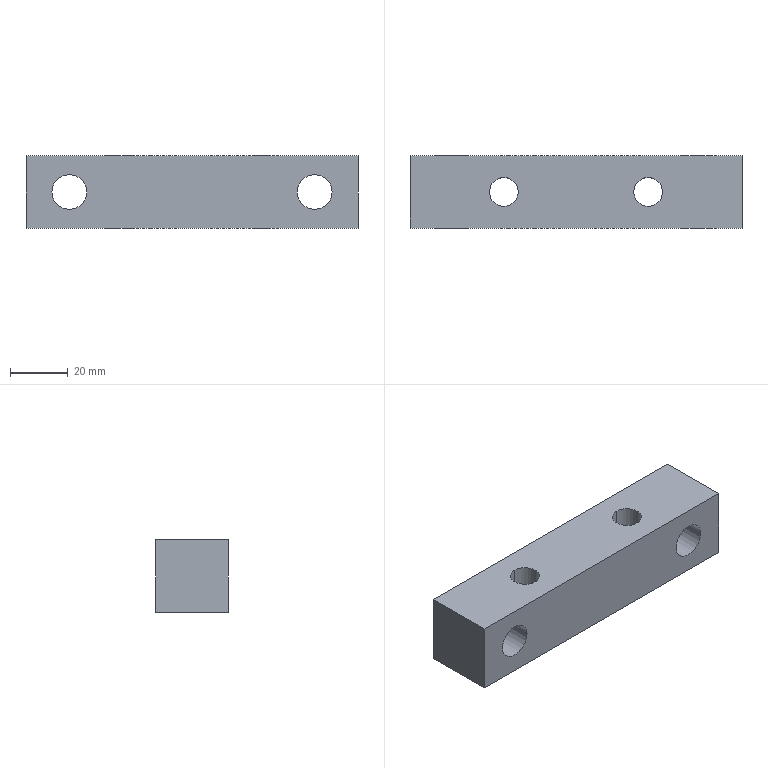Part | STEP file | J205-EBZ05-05-35 | 1 solid | 14 faces | box 115 x 25 x 25 mm | volume 62293 mm3 | cylinder 8 | plane 6 | commonest cylinder face diameters 10 x4 12 x4
STEP:
#1=CARTESIAN_POINT('',(84.,25.,12.5));
#2=VERTEX_POINT('',#1);
#3=CARTESIAN_POINT('',(96.,25.,12.5));
#4=VERTEX_POINT('',#3);
#5=CARTESIAN_POINT('',(90.,25.,12.5));
#6=DIRECTION('',(0.,-1.,0.));
#7=DIRECTION('',(1.,0.,0.));
#8=AXIS2_PLACEMENT_3D('',#5,#6,#7);
#9=CIRCLE('',#8,6.);
#10=EDGE_CURVE('',#2,#4,#9,.T.);
#11=ORIENTED_EDGE('',*,*,#10,.F.);
#12=CARTESIAN_POINT('',(84.,0.,12.5));
#13=VERTEX_POINT('',#12);
#14=CARTESIAN_POINT('',(84.,25.,12.5));
#15=DIRECTION('',(0.,-1.,0.));
#16=VECTOR('',#15,1000.);
#17=LINE('',#14,#16);
#18=EDGE_CURVE('',#2,#13,#17,.T.);
#19=ORIENTED_EDGE('',*,*,#18,.T.);
#20=CARTESIAN_POINT('',(96.,0.,12.5));
#21=VERTEX_POINT('',#20);
#22=CARTESIAN_POINT('',(90.,0.,12.5));
#23=DIRECTION('',(0.,1.,0.));
#24=DIRECTION('',(-1.,0.,0.));
#25=AXIS2_PLACEMENT_3D('',#22,#23,#24);
#26=CIRCLE('',#25,6.);
#27=EDGE_CURVE('',#21,#13,#26,.T.);
#28=ORIENTED_EDGE('',*,*,#27,.F.);
#29=CARTESIAN_POINT('',(96.,25.,12.5));
#30=DIRECTION('',(0.,-1.,0.));
#31=VECTOR('',#30,1000.);
#32=LINE('',#29,#31);
#33=EDGE_CURVE('',#4,#21,#32,.T.);
#34=ORIENTED_EDGE('',*,*,#33,.F.);
#35=EDGE_LOOP('',(#11,#19,#28,#34));
#36=FACE_OUTER_BOUND('',#35,.T.);
#37=CARTESIAN_POINT('',(90.,25.,12.5));
#38=DIRECTION('',(0.,-1.,0.));
#39=DIRECTION('',(1.,0.,0.));
#40=AXIS2_PLACEMENT_3D('',#37,#38,#39);
#41=CYLINDRICAL_SURFACE('',#40,6.);
#42=ADVANCED_FACE('',(#36),#41,.F.);
#43=CARTESIAN_POINT('',(-1.,25.,12.5));
#44=VERTEX_POINT('',#43);
#45=CARTESIAN_POINT('',(11.,25.,12.5));
#46=VERTEX_POINT('',#45);
#47=CARTESIAN_POINT('',(5.,25.,12.5));
#48=DIRECTION('',(0.,-1.,0.));
#49=DIRECTION('',(1.,0.,0.));
#50=AXIS2_PLACEMENT_3D('',#47,#48,#49);
#51=CIRCLE('',#50,6.);
#52=EDGE_CURVE('',#44,#46,#51,.T.);
#53=ORIENTED_EDGE('',*,*,#52,.F.);
#54=CARTESIAN_POINT('',(-1.,0.,12.5));
#55=VERTEX_POINT('',#54);
#56=CARTESIAN_POINT('',(-1.,25.,12.5));
#57=DIRECTION('',(0.,-1.,0.));
#58=VECTOR('',#57,1000.);
#59=LINE('',#56,#58);
#60=EDGE_CURVE('',#44,#55,#59,.T.);
#61=ORIENTED_EDGE('',*,*,#60,.T.);
#62=CARTESIAN_POINT('',(11.,0.,12.5));
#63=VERTEX_POINT('',#62);
#64=CARTESIAN_POINT('',(5.,0.,12.5));
#65=DIRECTION('',(0.,1.,0.));
#66=DIRECTION('',(-1.,0.,0.));
#67=AXIS2_PLACEMENT_3D('',#64,#65,#66);
#68=CIRCLE('',#67,6.);
#69=EDGE_CURVE('',#63,#55,#68,.T.);
#70=ORIENTED_EDGE('',*,*,#69,.F.);
#71=CARTESIAN_POINT('',(11.,25.,12.5));
#72=DIRECTION('',(0.,-1.,0.));
#73=VECTOR('',#72,1000.);
#74=LINE('',#71,#73);
#75=EDGE_CURVE('',#46,#63,#74,.T.);
#76=ORIENTED_EDGE('',*,*,#75,.F.);
#77=EDGE_LOOP('',(#53,#61,#70,#76));
#78=FACE_OUTER_BOUND('',#77,.T.);
#79=CARTESIAN_POINT('',(5.,25.,12.5));
#80=DIRECTION('',(0.,-1.,0.));
#81=DIRECTION('',(1.,0.,0.));
#82=AXIS2_PLACEMENT_3D('',#79,#80,#81);
#83=CYLINDRICAL_SURFACE('',#82,6.);
#84=ADVANCED_FACE('',(#78),#83,.F.);
#85=CARTESIAN_POINT('',(22.5,17.5,25.));
#86=VERTEX_POINT('',#85);
#87=CARTESIAN_POINT('',(22.5,7.5,25.));
#88=VERTEX_POINT('',#87);
#89=CARTESIAN_POINT('',(22.5,12.5,25.));
#90=DIRECTION('',(0.,0.,-1.));
#91=DIRECTION('',(0.,-1.,0.));
#92=AXIS2_PLACEMENT_3D('',#89,#90,#91);
#93=CIRCLE('',#92,5.);
#94=EDGE_CURVE('',#86,#88,#93,.T.);
#95=ORIENTED_EDGE('',*,*,#94,.F.);
#96=CARTESIAN_POINT('',(22.5,17.5,0.));
#97=VERTEX_POINT('',#96);
#98=CARTESIAN_POINT('',(22.5,17.5,25.));
#99=DIRECTION('',(0.,0.,-1.));
#100=VECTOR('',#99,1000.);
#101=LINE('',#98,#100);
#102=EDGE_CURVE('',#86,#97,#101,.T.);
#103=ORIENTED_EDGE('',*,*,#102,.T.);
#104=CARTESIAN_POINT('',(22.5,7.5,0.));
#105=VERTEX_POINT('',#104);
#106=CARTESIAN_POINT('',(22.5,12.5,0.));
#107=DIRECTION('',(0.,0.,1.));
#108=DIRECTION('',(0.,1.,0.));
#109=AXIS2_PLACEMENT_3D('',#106,#107,#108);
#110=CIRCLE('',#109,5.);
#111=EDGE_CURVE('',#105,#97,#110,.T.);
#112=ORIENTED_EDGE('',*,*,#111,.F.);
#113=CARTESIAN_POINT('',(22.5,7.5,25.));
#114=DIRECTION('',(0.,0.,-1.));
#115=VECTOR('',#114,1000.);
#116=LINE('',#113,#115);
#117=EDGE_CURVE('',#88,#105,#116,.T.);
#118=ORIENTED_EDGE('',*,*,#117,.F.);
#119=EDGE_LOOP('',(#95,#103,#112,#118));
#120=FACE_OUTER_BOUND('',#119,.T.);
#121=CARTESIAN_POINT('',(22.5,12.5,25.));
#122=DIRECTION('',(0.,0.,-1.));
#123=DIRECTION('',(0.,-1.,0.));
#124=AXIS2_PLACEMENT_3D('',#121,#122,#123);
#125=CYLINDRICAL_SURFACE('',#124,5.);
#126=ADVANCED_FACE('',(#120),#125,.F.);
#127=CARTESIAN_POINT('',(72.5,17.5,25.));
#128=VERTEX_POINT('',#127);
#129=CARTESIAN_POINT('',(72.5,7.5,25.));
#130=VERTEX_POINT('',#129);
#131=CARTESIAN_POINT('',(72.5,12.5,25.));
#132=DIRECTION('',(0.,0.,-1.));
#133=DIRECTION('',(0.,-1.,0.));
#134=AXIS2_PLACEMENT_3D('',#131,#132,#133);
#135=CIRCLE('',#134,5.);
#136=EDGE_CURVE('',#128,#130,#135,.T.);
#137=ORIENTED_EDGE('',*,*,#136,.F.);
#138=CARTESIAN_POINT('',(72.5,17.5,0.));
#139=VERTEX_POINT('',#138);
#140=CARTESIAN_POINT('',(72.5,17.5,25.));
#141=DIRECTION('',(0.,0.,-1.));
#142=VECTOR('',#141,1000.);
#143=LINE('',#140,#142);
#144=EDGE_CURVE('',#128,#139,#143,.T.);
#145=ORIENTED_EDGE('',*,*,#144,.T.);
#146=CARTESIAN_POINT('',(72.5,7.5,0.));
#147=VERTEX_POINT('',#146);
#148=CARTESIAN_POINT('',(72.5,12.5,0.));
#149=DIRECTION('',(0.,0.,1.));
#150=DIRECTION('',(0.,1.,0.));
#151=AXIS2_PLACEMENT_3D('',#148,#149,#150);
#152=CIRCLE('',#151,5.);
#153=EDGE_CURVE('',#147,#139,#152,.T.);
#154=ORIENTED_EDGE('',*,*,#153,.F.);
#155=CARTESIAN_POINT('',(72.5,7.5,25.));
#156=DIRECTION('',(0.,0.,-1.));
#157=VECTOR('',#156,1000.);
#158=LINE('',#155,#157);
#159=EDGE_CURVE('',#130,#147,#158,.T.);
#160=ORIENTED_EDGE('',*,*,#159,.F.);
#161=EDGE_LOOP('',(#137,#145,#154,#160));
#162=FACE_OUTER_BOUND('',#161,.T.);
#163=CARTESIAN_POINT('',(72.5,12.5,25.));
#164=DIRECTION('',(0.,0.,-1.));
#165=DIRECTION('',(0.,-1.,0.));
#166=AXIS2_PLACEMENT_3D('',#163,#164,#165);
#167=CYLINDRICAL_SURFACE('',#166,5.);
#168=ADVANCED_FACE('',(#162),#167,.F.);
#169=CARTESIAN_POINT('',(90.,25.,12.5));
#170=DIRECTION('',(0.,-1.,0.));
#171=DIRECTION('',(1.,0.,0.));
#172=AXIS2_PLACEMENT_3D('',#169,#170,#171);
#173=CIRCLE('',#172,6.);
#174=EDGE_CURVE('',#4,#2,#173,.T.);
#175=ORIENTED_EDGE('',*,*,#174,.T.);
#176=ORIENTED_EDGE('',*,*,#10,.T.);
#177=EDGE_LOOP('',(#175,#176));
#178=FACE_BOUND('',#177,.T.);
#179=CARTESIAN_POINT('',(5.,25.,12.5));
#180=DIRECTION('',(0.,-1.,0.));
#181=DIRECTION('',(1.,0.,0.));
#182=AXIS2_PLACEMENT_3D('',#179,#180,#181);
#183=CIRCLE('',#182,6.);
#184=EDGE_CURVE('',#46,#44,#183,.T.);
#185=ORIENTED_EDGE('',*,*,#184,.T.);
#186=ORIENTED_EDGE('',*,*,#52,.T.);
#187=EDGE_LOOP('',(#185,#186));
#188=FACE_BOUND('',#187,.T.);
#189=CARTESIAN_POINT('',(-10.,25.,0.));
#190=VERTEX_POINT('',#189);
#191=CARTESIAN_POINT('',(105.,25.,0.));
#192=VERTEX_POINT('',#191);
#193=CARTESIAN_POINT('',(47.5,25.,0.));
#194=DIRECTION('',(1.,0.,0.));
#195=VECTOR('',#194,1000.);
#196=LINE('',#193,#195);
#197=EDGE_CURVE('',#190,#192,#196,.T.);
#198=ORIENTED_EDGE('',*,*,#197,.F.);
#199=CARTESIAN_POINT('',(-10.,25.,25.));
#200=VERTEX_POINT('',#199);
#201=CARTESIAN_POINT('',(-10.,25.,12.5));
#202=DIRECTION('',(0.,0.,-1.));
#203=VECTOR('',#202,1000.);
#204=LINE('',#201,#203);
#205=EDGE_CURVE('',#200,#190,#204,.T.);
#206=ORIENTED_EDGE('',*,*,#205,.F.);
#207=CARTESIAN_POINT('',(105.,25.,25.));
#208=VERTEX_POINT('',#207);
#209=CARTESIAN_POINT('',(47.5,25.,25.));
#210=DIRECTION('',(-1.,0.,0.));
#211=VECTOR('',#210,1000.);
#212=LINE('',#209,#211);
#213=EDGE_CURVE('',#208,#200,#212,.T.);
#214=ORIENTED_EDGE('',*,*,#213,.F.);
#215=CARTESIAN_POINT('',(105.,25.,12.5));
#216=DIRECTION('',(0.,0.,1.));
#217=VECTOR('',#216,1000.);
#218=LINE('',#215,#217);
#219=EDGE_CURVE('',#192,#208,#218,.T.);
#220=ORIENTED_EDGE('',*,*,#219,.F.);
#221=EDGE_LOOP('',(#198,#206,#214,#220));
#222=FACE_OUTER_BOUND('',#221,.T.);
#223=CARTESIAN_POINT('',(47.5,25.,12.5));
#224=DIRECTION('',(0.,1.,0.));
#225=DIRECTION('',(-1.,0.,0.));
#226=AXIS2_PLACEMENT_3D('',#223,#224,#225);
#227=PLANE('',#226);
#228=ADVANCED_FACE('',(#178,#188,#222),#227,.T.);
#229=ORIENTED_EDGE('',*,*,#111,.T.);
#230=CARTESIAN_POINT('',(22.5,12.5,0.));
#231=DIRECTION('',(0.,0.,1.));
#232=DIRECTION('',(0.,1.,0.));
#233=AXIS2_PLACEMENT_3D('',#230,#231,#232);
#234=CIRCLE('',#233,5.);
#235=EDGE_CURVE('',#97,#105,#234,.T.);
#236=ORIENTED_EDGE('',*,*,#235,.T.);
#237=EDGE_LOOP('',(#229,#236));
#238=FACE_BOUND('',#237,.T.);
#239=ORIENTED_EDGE('',*,*,#153,.T.);
#240=CARTESIAN_POINT('',(72.5,12.5,0.));
#241=DIRECTION('',(0.,0.,1.));
#242=DIRECTION('',(0.,1.,0.));
#243=AXIS2_PLACEMENT_3D('',#240,#241,#242);
#244=CIRCLE('',#243,5.);
#245=EDGE_CURVE('',#139,#147,#244,.T.);
#246=ORIENTED_EDGE('',*,*,#245,.T.);
#247=EDGE_LOOP('',(#239,#246));
#248=FACE_BOUND('',#247,.T.);
#249=CARTESIAN_POINT('',(-10.,0.,0.));
#250=VERTEX_POINT('',#249);
#251=CARTESIAN_POINT('',(-10.,0.,0.));
#252=DIRECTION('',(0.,1.,0.));
#253=VECTOR('',#252,1000.);
#254=LINE('',#251,#253);
#255=EDGE_CURVE('',#250,#190,#254,.T.);
#256=ORIENTED_EDGE('',*,*,#255,.T.);
#257=ORIENTED_EDGE('',*,*,#197,.T.);
#258=CARTESIAN_POINT('',(105.,0.,0.));
#259=VERTEX_POINT('',#258);
#260=CARTESIAN_POINT('',(105.,0.,0.));
#261=DIRECTION('',(0.,1.,0.));
#262=VECTOR('',#261,1000.);
#263=LINE('',#260,#262);
#264=EDGE_CURVE('',#259,#192,#263,.T.);
#265=ORIENTED_EDGE('',*,*,#264,.F.);
#266=CARTESIAN_POINT('',(47.5,0.,0.));
#267=DIRECTION('',(-1.,0.,0.));
#268=VECTOR('',#267,1000.);
#269=LINE('',#266,#268);
#270=EDGE_CURVE('',#259,#250,#269,.T.);
#271=ORIENTED_EDGE('',*,*,#270,.T.);
#272=EDGE_LOOP('',(#256,#257,#265,#271));
#273=FACE_OUTER_BOUND('',#272,.T.);
#274=CARTESIAN_POINT('',(47.5,0.,0.));
#275=DIRECTION('',(0.,0.,-1.));
#276=DIRECTION('',(0.,-1.,0.));
#277=AXIS2_PLACEMENT_3D('',#274,#275,#276);
#278=PLANE('',#277);
#279=ADVANCED_FACE('',(#238,#248,#273),#278,.T.);
#280=ORIENTED_EDGE('',*,*,#264,.T.);
#281=ORIENTED_EDGE('',*,*,#219,.T.);
#282=CARTESIAN_POINT('',(105.,0.,25.));
#283=VERTEX_POINT('',#282);
#284=CARTESIAN_POINT('',(105.,0.,25.));
#285=DIRECTION('',(0.,1.,0.));
#286=VECTOR('',#285,1000.);
#287=LINE('',#284,#286);
#288=EDGE_CURVE('',#283,#208,#287,.T.);
#289=ORIENTED_EDGE('',*,*,#288,.F.);
#290=CARTESIAN_POINT('',(105.,0.,12.5));
#291=DIRECTION('',(0.,0.,-1.));
#292=VECTOR('',#291,1000.);
#293=LINE('',#290,#292);
#294=EDGE_CURVE('',#283,#259,#293,.T.);
#295=ORIENTED_EDGE('',*,*,#294,.T.);
#296=EDGE_LOOP('',(#280,#281,#289,#295));
#297=FACE_OUTER_BOUND('',#296,.T.);
#298=CARTESIAN_POINT('',(105.,0.,12.5));
#299=DIRECTION('',(1.,0.,0.));
#300=DIRECTION('',(0.,1.,0.));
#301=AXIS2_PLACEMENT_3D('',#298,#299,#300);
#302=PLANE('',#301);
#303=ADVANCED_FACE('',(#297),#302,.T.);
#304=CARTESIAN_POINT('',(22.5,12.5,25.));
#305=DIRECTION('',(0.,0.,-1.));
#306=DIRECTION('',(0.,-1.,0.));
#307=AXIS2_PLACEMENT_3D('',#304,#305,#306);
#308=CIRCLE('',#307,5.);
#309=EDGE_CURVE('',#88,#86,#308,.T.);
#310=ORIENTED_EDGE('',*,*,#309,.T.);
#311=ORIENTED_EDGE('',*,*,#94,.T.);
#312=EDGE_LOOP('',(#310,#311));
#313=FACE_BOUND('',#312,.T.);
#314=CARTESIAN_POINT('',(72.5,12.5,25.));
#315=DIRECTION('',(0.,0.,-1.));
#316=DIRECTION('',(0.,-1.,0.));
#317=AXIS2_PLACEMENT_3D('',#314,#315,#316);
#318=CIRCLE('',#317,5.);
#319=EDGE_CURVE('',#130,#128,#318,.T.);
#320=ORIENTED_EDGE('',*,*,#319,.T.);
#321=ORIENTED_EDGE('',*,*,#136,.T.);
#322=EDGE_LOOP('',(#320,#321));
#323=FACE_BOUND('',#322,.T.);
#324=ORIENTED_EDGE('',*,*,#288,.T.);
#325=ORIENTED_EDGE('',*,*,#213,.T.);
#326=CARTESIAN_POINT('',(-10.,0.,25.));
#327=VERTEX_POINT('',#326);
#328=CARTESIAN_POINT('',(-10.,0.,25.));
#329=DIRECTION('',(0.,1.,0.));
#330=VECTOR('',#329,1000.);
#331=LINE('',#328,#330);
#332=EDGE_CURVE('',#327,#200,#331,.T.);
#333=ORIENTED_EDGE('',*,*,#332,.F.);
#334=CARTESIAN_POINT('',(47.5,0.,25.));
#335=DIRECTION('',(1.,0.,0.));
#336=VECTOR('',#335,1000.);
#337=LINE('',#334,#336);
#338=EDGE_CURVE('',#327,#283,#337,.T.);
#339=ORIENTED_EDGE('',*,*,#338,.T.);
#340=EDGE_LOOP('',(#324,#325,#333,#339));
#341=FACE_OUTER_BOUND('',#340,.T.);
#342=CARTESIAN_POINT('',(47.5,0.,25.));
#343=DIRECTION('',(0.,0.,1.));
#344=DIRECTION('',(0.,1.,0.));
#345=AXIS2_PLACEMENT_3D('',#342,#343,#344);
#346=PLANE('',#345);
#347=ADVANCED_FACE('',(#313,#323,#341),#346,.T.);
#348=ORIENTED_EDGE('',*,*,#27,.T.);
#349=CARTESIAN_POINT('',(90.,0.,12.5));
#350=DIRECTION('',(0.,1.,0.));
#351=DIRECTION('',(-1.,0.,0.));
#352=AXIS2_PLACEMENT_3D('',#349,#350,#351);
#353=CIRCLE('',#352,6.);
#354=EDGE_CURVE('',#13,#21,#353,.T.);
#355=ORIENTED_EDGE('',*,*,#354,.T.);
#356=EDGE_LOOP('',(#348,#355));
#357=FACE_BOUND('',#356,.T.);
#358=ORIENTED_EDGE('',*,*,#69,.T.);
#359=CARTESIAN_POINT('',(5.,0.,12.5));
#360=DIRECTION('',(0.,1.,0.));
#361=DIRECTION('',(-1.,0.,0.));
#362=AXIS2_PLACEMENT_3D('',#359,#360,#361);
#363=CIRCLE('',#362,6.);
#364=EDGE_CURVE('',#55,#63,#363,.T.);
#365=ORIENTED_EDGE('',*,*,#364,.T.);
#366=EDGE_LOOP('',(#358,#365));
#367=FACE_BOUND('',#366,.T.);
#368=CARTESIAN_POINT('',(-10.,0.,12.5));
#369=DIRECTION('',(0.,0.,1.));
#370=VECTOR('',#369,1000.);
#371=LINE('',#368,#370);
#372=EDGE_CURVE('',#250,#327,#371,.T.);
#373=ORIENTED_EDGE('',*,*,#372,.F.);
#374=ORIENTED_EDGE('',*,*,#270,.F.);
#375=ORIENTED_EDGE('',*,*,#294,.F.);
#376=ORIENTED_EDGE('',*,*,#338,.F.);
#377=EDGE_LOOP('',(#373,#374,#375,#376));
#378=FACE_OUTER_BOUND('',#377,.T.);
#379=CARTESIAN_POINT('',(47.5,0.,12.5));
#380=DIRECTION('',(0.,-1.,0.));
#381=DIRECTION('',(1.,0.,0.));
#382=AXIS2_PLACEMENT_3D('',#379,#380,#381);
#383=PLANE('',#382);
#384=ADVANCED_FACE('',(#357,#367,#378),#383,.T.);
#385=ORIENTED_EDGE('',*,*,#372,.T.);
#386=ORIENTED_EDGE('',*,*,#332,.T.);
#387=ORIENTED_EDGE('',*,*,#205,.T.);
#388=ORIENTED_EDGE('',*,*,#255,.F.);
#389=EDGE_LOOP('',(#385,#386,#387,#388));
#390=FACE_OUTER_BOUND('',#389,.T.);
#391=CARTESIAN_POINT('',(-10.,0.,12.5));
#392=DIRECTION('',(-1.,0.,0.));
#393=DIRECTION('',(0.,-1.,0.));
#394=AXIS2_PLACEMENT_3D('',#391,#392,#393);
#395=PLANE('',#394);
#396=ADVANCED_FACE('',(#390),#395,.T.);
#397=ORIENTED_EDGE('',*,*,#144,.F.);
#398=ORIENTED_EDGE('',*,*,#319,.F.);
#399=ORIENTED_EDGE('',*,*,#159,.T.);
#400=ORIENTED_EDGE('',*,*,#245,.F.);
#401=EDGE_LOOP('',(#397,#398,#399,#400));
#402=FACE_OUTER_BOUND('',#401,.T.);
#403=CARTESIAN_POINT('',(72.5,12.5,25.));
#404=DIRECTION('',(0.,0.,-1.));
#405=DIRECTION('',(0.,-1.,0.));
#406=AXIS2_PLACEMENT_3D('',#403,#404,#405);
#407=CYLINDRICAL_SURFACE('',#406,5.);
#408=ADVANCED_FACE('',(#402),#407,.F.);
#409=ORIENTED_EDGE('',*,*,#102,.F.);
#410=ORIENTED_EDGE('',*,*,#309,.F.);
#411=ORIENTED_EDGE('',*,*,#117,.T.);
#412=ORIENTED_EDGE('',*,*,#235,.F.);
#413=EDGE_LOOP('',(#409,#410,#411,#412));
#414=FACE_OUTER_BOUND('',#413,.T.);
#415=CARTESIAN_POINT('',(22.5,12.5,25.));
#416=DIRECTION('',(0.,0.,-1.));
#417=DIRECTION('',(0.,-1.,0.));
#418=AXIS2_PLACEMENT_3D('',#415,#416,#417);
#419=CYLINDRICAL_SURFACE('',#418,5.);
#420=ADVANCED_FACE('',(#414),#419,.F.);
#421=ORIENTED_EDGE('',*,*,#60,.F.);
#422=ORIENTED_EDGE('',*,*,#184,.F.);
#423=ORIENTED_EDGE('',*,*,#75,.T.);
#424=ORIENTED_EDGE('',*,*,#364,.F.);
#425=EDGE_LOOP('',(#421,#422,#423,#424));
#426=FACE_OUTER_BOUND('',#425,.T.);
#427=CARTESIAN_POINT('',(5.,25.,12.5));
#428=DIRECTION('',(0.,-1.,0.));
#429=DIRECTION('',(1.,0.,0.));
#430=AXIS2_PLACEMENT_3D('',#427,#428,#429);
#431=CYLINDRICAL_SURFACE('',#430,6.);
#432=ADVANCED_FACE('',(#426),#431,.F.);
#433=ORIENTED_EDGE('',*,*,#18,.F.);
#434=ORIENTED_EDGE('',*,*,#174,.F.);
#435=ORIENTED_EDGE('',*,*,#33,.T.);
#436=ORIENTED_EDGE('',*,*,#354,.F.);
#437=EDGE_LOOP('',(#433,#434,#435,#436));
#438=FACE_OUTER_BOUND('',#437,.T.);
#439=CARTESIAN_POINT('',(90.,25.,12.5));
#440=DIRECTION('',(0.,-1.,0.));
#441=DIRECTION('',(1.,0.,0.));
#442=AXIS2_PLACEMENT_3D('',#439,#440,#441);
#443=CYLINDRICAL_SURFACE('',#442,6.);
#444=ADVANCED_FACE('',(#438),#443,.F.);
#445=CLOSED_SHELL('',(#42,#84,#126,#168,#228,#279,#303,#347,#384,#396,#408,#420,#432,#444));
#446=MANIFOLD_SOLID_BREP('',#445);
#447=CARTESIAN_POINT('',(0.,0.,0.));
#448=DIRECTION('',(0.,0.,1.));
#449=DIRECTION('',(1.,0.,0.));
#450=AXIS2_PLACEMENT_3D('',#447,#448,#449);
#451=(LENGTH_UNIT()NAMED_UNIT(*)SI_UNIT(.MILLI.,.METRE.));
#452=UNCERTAINTY_MEASURE_WITH_UNIT(LENGTH_MEASURE(0.00001),#451,'','');
#453=(NAMED_UNIT(*)PLANE_ANGLE_UNIT()SI_UNIT($,.RADIAN.));
#454=(NAMED_UNIT(*)SI_UNIT($,.STERADIAN.)SOLID_ANGLE_UNIT());
#455=(GEOMETRIC_REPRESENTATION_CONTEXT(3)GLOBAL_UNCERTAINTY_ASSIGNED_CONTEXT((#452))GLOBAL_UNIT_ASSIGNED_CONTEXT((#451,#453,#454))REPRESENTATION_CONTEXT('',''));
#456=ADVANCED_BREP_SHAPE_REPRESENTATION('',(#446,#450),#455);